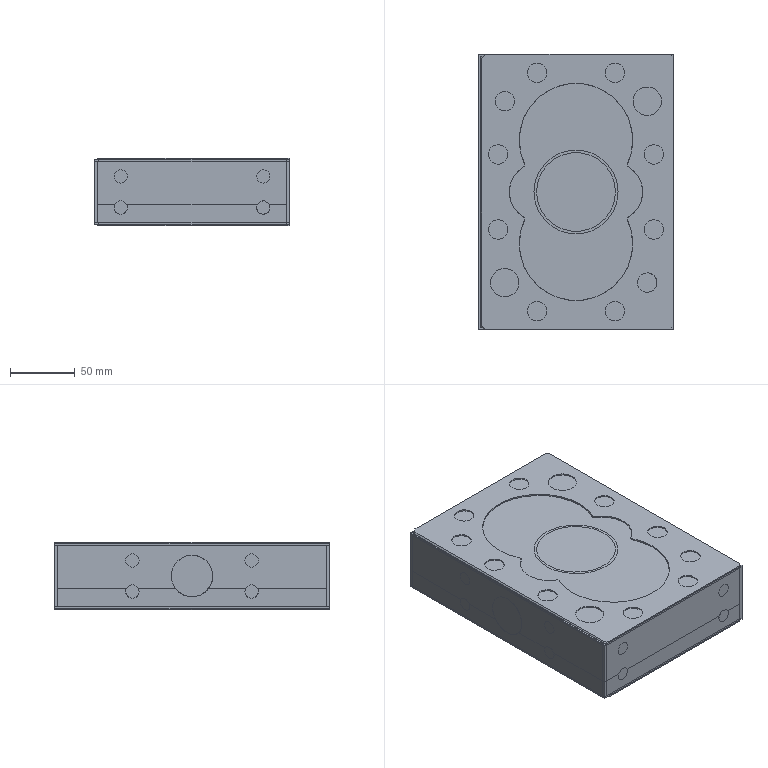NC program | NX | posted with a generic post | part box 150.2 x 212.2 x 52.4 mm
Lines 10319 to 11045 of 152230:
(孔铣开粗 , TOOL : D17R0.8圆鼻飞刀)
N20612 T03 M6
N20614 /M1
N20616 G54
N20618 G17 G0 G90 X-70. Y55. S1500 M3
N20620 G43 Z100. H3
N20622 Z1.2
N20624 G94 G1 Z0.2 F960.
N20626 G3 X-68.7 Y56.3 R1.3
N20628 X-70. Y57.6 R1.3
N20630 X-70. Y57.6 Z0. I0. J-2.6 F1200.
N20632 X-70. Y57.6 Z-0.2 I0. J-2.6
N20634 X-70. Y57.6 Z-0.4 I0. J-2.6
N20636 X-70. Y57.6 Z-0.6 I0. J-2.6
N20638 X-70. Y57.6 Z-0.8 I0. J-2.6
N20640 X-70. Y57.6 Z-1. I0. J-2.6
N20642 X-70. Y57.6 Z-1.2 I0. J-2.6
N20644 X-70. Y57.6 Z-1.4 I0. J-2.6
N20646 X-70. Y57.6 Z-1.6 I0. J-2.6
N20648 X-70. Y57.6 Z-1.8 I0. J-2.6
N20650 X-70. Y57.6 Z-2. I0. J-2.6
N20652 X-70. Y57.6 Z-2.2 I0. J-2.6
N20654 X-70. Y57.6 Z-2.4 I0. J-2.6
N20656 X-70. Y57.6 Z-2.6 I0. J-2.6
N20658 X-70. Y57.6 Z-2.8 I0. J-2.6
N20660 X-70. Y57.6 Z-3. I0. J-2.6
N20662 X-70. Y57.6 Z-3.2 I0. J-2.6
N20664 X-70. Y57.6 Z-3.4 I0. J-2.6
N20666 X-70. Y57.6 Z-3.6 I0. J-2.6
N20668 X-70. Y57.6 Z-3.8 I0. J-2.6
N20670 X-70. Y57.6 Z-4. I0. J-2.6
N20672 X-70. Y57.6 Z-4.2 I0. J-2.6
N20674 X-70. Y57.6 Z-4.4 I0. J-2.6
N20676 X-70. Y57.6 Z-4.6 I0. J-2.6
N20678 X-70. Y57.6 Z-4.8 I0. J-2.6
N20680 X-70. Y57.6 Z-5. I0. J-2.6
N20682 X-70. Y57.6 Z-5.2 I0. J-2.6
N20684 X-70. Y57.6 Z-5.4 I0. J-2.6
N20686 X-70. Y57.6 Z-5.6 I0. J-2.6
N20688 X-70. Y57.6 Z-5.8 I0. J-2.6
N20690 X-70. Y57.6 Z-6. I0. J-2.6
N20692 X-70. Y57.6 Z-6.2 I0. J-2.6
N20694 X-70. Y57.6 Z-6.4 I0. J-2.6
N20696 X-70. Y57.6 Z-6.6 I0. J-2.6
N20698 X-70. Y57.6 Z-6.8 I0. J-2.6
N20700 X-70. Y57.6 Z-7. I0. J-2.6
N20702 X-70. Y57.6 Z-7.2 I0. J-2.6
N20704 X-70. Y57.6 Z-7.4 I0. J-2.6
N20706 X-70. Y57.6 Z-7.6 I0. J-2.6
N20708 X-70. Y57.6 Z-7.8 I0. J-2.6
N20710 X-70. Y57.6 Z-8. I0. J-2.6
N20712 X-70. Y57.6 Z-8.2 I0. J-2.6
N20714 X-70. Y57.6 Z-8.4 I0. J-2.6
N20716 X-70. Y57.6 Z-8.6 I0. J-2.6
N20718 X-70. Y57.6 Z-8.8 I0. J-2.6
N20720 X-70. Y57.6 Z-9. I0. J-2.6
N20722 X-70. Y57.6 Z-9.2 I0. J-2.6
N20724 X-70. Y57.6 Z-9.4 I0. J-2.6
N20726 X-70. Y57.6 Z-9.6 I0. J-2.6
N20728 X-70. Y57.6 Z-9.8 I0. J-2.6
N20730 X-70. Y57.6 Z-10. I0. J-2.6
N20732 X-70. Y57.6 Z-10.2 I0. J-2.6
N20734 X-70. Y57.6 Z-10.4 I0. J-2.6
N20736 X-70. Y57.6 Z-10.6 I0. J-2.6
N20738 X-70. Y57.6 Z-10.8 I0. J-2.6
N20740 X-70. Y57.6 Z-11. I0. J-2.6
N20742 X-70. Y57.6 Z-11.2 I0. J-2.6
N20744 X-70. Y57.6 Z-11.4 I0. J-2.6
N20746 X-70. Y57.6 Z-11.6 I0. J-2.6
N20748 X-70. Y57.6 Z-11.8 I0. J-2.6
N20750 X-70. Y57.6 Z-12. I0. J-2.6
N20752 X-70. Y57.6 Z-12.2 I0. J-2.6
N20754 X-70. Y57.6 Z-12.4 I0. J-2.6
N20756 X-70. Y57.6 Z-12.6 I0. J-2.6
N20758 X-70. Y57.6 Z-12.8 I0. J-2.6
N20760 X-70. Y57.6 Z-13. I0. J-2.6
N20762 X-70. Y57.6 Z-13.2 I0. J-2.6
N20764 X-70. Y57.6 Z-13.4 I0. J-2.6
N20766 X-70. Y57.6 Z-13.6 I0. J-2.6
N20768 X-70. Y57.6 Z-13.8 I0. J-2.6
N20770 X-70. Y57.6 Z-14. I0. J-2.6
N20772 X-70. Y57.6 Z-14.2 I0. J-2.6
N20774 X-70. Y57.6 Z-14.4 I0. J-2.6
N20776 X-70. Y57.6 Z-14.6 I0. J-2.6
N20778 X-70. Y57.6 Z-14.8 I0. J-2.6
N20780 X-70. Y57.6 Z-15. I0. J-2.6
N20782 X-70. Y57.6 Z-15.2 I0. J-2.6
N20784 X-70. Y57.6 Z-15.4 I0. J-2.6
N20786 X-70. Y57.6 Z-15.6 I0. J-2.6
N20788 X-70. Y57.6 Z-15.8 I0. J-2.6
N20790 X-70. Y57.6 Z-16. I0. J-2.6
N20792 X-70. Y57.6 Z-16.2 I0. J-2.6
N20794 X-70. Y57.6 Z-16.4 I0. J-2.6
N20796 X-70. Y57.6 Z-16.6 I0. J-2.6
N20798 X-70. Y57.6 Z-16.8 I0. J-2.6
N20800 X-70. Y57.6 Z-17. I0. J-2.6
N20802 X-70. Y57.6 Z-17.2 I0. J-2.6
N20804 X-70. Y57.6 Z-17.4 I0. J-2.6
N20806 X-70. Y57.6 Z-17.6 I0. J-2.6
N20808 X-70. Y57.6 Z-17.8 I0. J-2.6
N20810 X-70. Y57.6 Z-18. I0. J-2.6
N20812 X-70. Y57.6 Z-18.2 I0. J-2.6
N20814 X-70. Y57.6 Z-18.4 I0. J-2.6
N20816 X-70. Y57.6 Z-18.6 I0. J-2.6
N20818 X-70. Y57.6 Z-18.8 I0. J-2.6
N20820 X-70. Y57.6 Z-19. I0. J-2.6
N20822 X-70. Y57.6 Z-19.2 I0. J-2.6
N20824 X-70. Y57.6 Z-19.4 I0. J-2.6
N20826 X-70. Y57.6 Z-19.6 I0. J-2.6
N20828 X-70. Y57.6 Z-19.8 I0. J-2.6
N20830 X-70. Y57.6 Z-20. I0. J-2.6
N20832 X-70. Y57.6 Z-20.2 I0. J-2.6
N20834 X-70. Y57.6 Z-20.4 I0. J-2.6
N20836 X-70. Y57.6 Z-20.6 I0. J-2.6
N20838 X-70. Y57.6 Z-20.8 I0. J-2.6
N20840 X-70. Y57.6 Z-21. I0. J-2.6
N20842 X-70. Y57.6 Z-21.2 I0. J-2.6
N20844 X-70. Y57.6 Z-21.4 I0. J-2.6
N20846 X-70. Y57.6 Z-21.6 I0. J-2.6
N20848 X-70. Y57.6 Z-21.8 I0. J-2.6
N20850 X-70. Y57.6 Z-22. I0. J-2.6
N20852 X-70. Y57.6 Z-22.2 I0. J-2.6
N20854 X-70. Y57.6 Z-22.4 I0. J-2.6
N20856 X-70. Y57.6 Z-22.6 I0. J-2.6
N20858 X-70. Y57.6 Z-22.8 I0. J-2.6
N20860 X-70. Y57.6 Z-23. I0. J-2.6
N20862 X-70. Y57.6 Z-23.2 I0. J-2.6
N20864 X-70. Y57.6 Z-23.4 I0. J-2.6
N20866 X-70. Y57.6 Z-23.6 I0. J-2.6
N20868 X-70. Y57.6 Z-23.8 I0. J-2.6
N20870 X-70. Y57.6 Z-24. I0. J-2.6
N20872 X-70. Y57.6 Z-24.2 I0. J-2.6
N20874 X-70. Y57.6 Z-24.4 I0. J-2.6
N20876 X-70. Y57.6 Z-24.6 I0. J-2.6
N20878 X-70. Y57.6 Z-24.8 I0. J-2.6
N20880 X-70. Y57.6 Z-25. I0. J-2.6
N20882 X-70. Y57.6 Z-25.2 I0. J-2.6
N20884 X-70. Y57.6 Z-25.4 I0. J-2.6
N20886 X-70. Y57.6 Z-25.6 I0. J-2.6
N20888 X-70. Y57.6 Z-25.8 I0. J-2.6
N20890 X-70. Y57.6 Z-26. I0. J-2.6
N20892 X-70. Y57.6 Z-26.2 I0. J-2.6
N20894 X-70. Y57.6 Z-26.4 I0. J-2.6
N20896 X-70. Y57.6 Z-26.6 I0. J-2.6
N20898 X-70. Y57.6 Z-26.8 I0. J-2.6
N20900 X-70. Y57.6 Z-27. I0. J-2.6
N20902 X-70. Y57.6 Z-27.2 I0. J-2.6
N20904 X-70. Y57.6 Z-27.4 I0. J-2.6
N20906 X-70. Y57.6 Z-27.6 I0. J-2.6
N20908 X-70. Y57.6 Z-27.8 I0. J-2.6
N20910 X-70. Y57.6 Z-28. I0. J-2.6
N20912 X-70. Y57.6 Z-28.2 I0. J-2.6
N20914 X-70. Y57.6 Z-28.4 I0. J-2.6
N20916 X-70. Y57.6 Z-28.6 I0. J-2.6
N20918 X-70. Y57.6 Z-28.8 I0. J-2.6
N20920 X-70. Y57.6 Z-29. I0. J-2.6
N20922 X-70. Y57.6 Z-29.2 I0. J-2.6
N20924 X-70. Y57.6 Z-29.4 I0. J-2.6
N20926 X-70. Y57.6 Z-29.6 I0. J-2.6
N20928 X-70. Y57.6 Z-29.8 I0. J-2.6
N20930 X-70. Y57.6 Z-30. I0. J-2.6
N20932 X-70. Y57.6 Z-30.2 I0. J-2.6
N20934 X-70. Y57.6 Z-30.4 I0. J-2.6
N20936 X-70. Y57.6 Z-30.6 I0. J-2.6
N20938 X-70. Y57.6 Z-30.8 I0. J-2.6
N20940 X-70. Y57.6 Z-31. I0. J-2.6
N20942 X-70. Y57.6 Z-31.2 I0. J-2.6
N20944 X-70. Y57.6 Z-31.4 I0. J-2.6
N20946 X-70. Y57.6 Z-31.6 I0. J-2.6
N20948 X-70. Y57.6 Z-31.8 I0. J-2.6
N20950 X-70. Y57.6 Z-32. I0. J-2.6
N20952 X-70. Y57.6 Z-32.2 I0. J-2.6
N20954 X-70. Y57.6 Z-32.4 I0. J-2.6
N20956 X-70. Y57.6 Z-32.6 I0. J-2.6
N20958 X-70. Y57.6 Z-32.8 I0. J-2.6
N20960 X-70. Y57.6 Z-33. I0. J-2.6
N20962 X-70. Y57.6 Z-33.2 I0. J-2.6
N20964 X-70. Y57.6 Z-33.4 I0. J-2.6
N20966 X-70. Y57.6 Z-33.6 I0. J-2.6
N20968 X-70. Y57.6 Z-33.8 I0. J-2.6
N20970 X-70. Y57.6 Z-34. I0. J-2.6
N20972 X-70. Y57.6 Z-34.2 I0. J-2.6
N20974 X-70. Y57.6 Z-34.4 I0. J-2.6
N20976 X-70. Y57.6 Z-34.6 I0. J-2.6
N20978 X-70. Y57.6 Z-34.8 I0. J-2.6
N20980 X-70. Y57.6 Z-35. I0. J-2.6
N20982 X-72.6 Y55. R2.6
N20984 X-70. Y57.6 R-2.6
N20986 X-71.3 Y56.3 R1.3
N20988 X-70. Y55. R1.3
N20990 G0 Z100.
N20992 X70. Y-55.
N20994 Z1.2
N20996 G1 Z0.2 F960.
N20998 G3 X71.3 Y-53.7 R1.3
N21000 X70. Y-52.4 R1.3
N21002 X70. Y-52.4 Z0. I0. J-2.6 F1200.
N21004 X70. Y-52.4 Z-0.2 I0. J-2.6
N21006 X70. Y-52.4 Z-0.4 I0. J-2.6
N21008 X70. Y-52.4 Z-0.6 I0. J-2.6
N21010 X70. Y-52.4 Z-0.8 I0. J-2.6
N21012 X70. Y-52.4 Z-1. I0. J-2.6
N21014 X70. Y-52.4 Z-1.2 I0. J-2.6
N21016 X70. Y-52.4 Z-1.4 I0. J-2.6
N21018 X70. Y-52.4 Z-1.6 I0. J-2.6
N21020 X70. Y-52.4 Z-1.8 I0. J-2.6
N21022 X70. Y-52.4 Z-2. I0. J-2.6
N21024 X70. Y-52.4 Z-2.2 I0. J-2.6
N21026 X70. Y-52.4 Z-2.4 I0. J-2.6
N21028 X70. Y-52.4 Z-2.6 I0. J-2.6
N21030 X70. Y-52.4 Z-2.8 I0. J-2.6
N21032 X70. Y-52.4 Z-3. I0. J-2.6
N21034 X70. Y-52.4 Z-3.2 I0. J-2.6
N21036 X70. Y-52.4 Z-3.4 I0. J-2.6
N21038 X70. Y-52.4 Z-3.6 I0. J-2.6
N21040 X70. Y-52.4 Z-3.8 I0. J-2.6
N21042 X70. Y-52.4 Z-4. I0. J-2.6
N21044 X70. Y-52.4 Z-4.2 I0. J-2.6
N21046 X70. Y-52.4 Z-4.4 I0. J-2.6
N21048 X70. Y-52.4 Z-4.6 I0. J-2.6
N21050 X70. Y-52.4 Z-4.8 I0. J-2.6
N21052 X70. Y-52.4 Z-5. I0. J-2.6
N21054 X70. Y-52.4 Z-5.2 I0. J-2.6
N21056 X70. Y-52.4 Z-5.4 I0. J-2.6
N21058 X70. Y-52.4 Z-5.6 I0. J-2.6
N21060 X70. Y-52.4 Z-5.8 I0. J-2.6
N21062 X70. Y-52.4 Z-6. I0. J-2.6
N21064 X70. Y-52.4 Z-6.2 I0. J-2.6
N21066 X70. Y-52.4 Z-6.4 I0. J-2.6
N21068 X70. Y-52.4 Z-6.6 I0. J-2.6
N21070 X70. Y-52.4 Z-6.8 I0. J-2.6
N21072 X70. Y-52.4 Z-7. I0. J-2.6
N21074 X70. Y-52.4 Z-7.2 I0. J-2.6
N21076 X70. Y-52.4 Z-7.4 I0. J-2.6
N21078 X70. Y-52.4 Z-7.6 I0. J-2.6
N21080 X70. Y-52.4 Z-7.8 I0. J-2.6
N21082 X70. Y-52.4 Z-8. I0. J-2.6
N21084 X70. Y-52.4 Z-8.2 I0. J-2.6
N21086 X70. Y-52.4 Z-8.4 I0. J-2.6
N21088 X70. Y-52.4 Z-8.6 I0. J-2.6
N21090 X70. Y-52.4 Z-8.8 I0. J-2.6
N21092 X70. Y-52.4 Z-9. I0. J-2.6
N21094 X70. Y-52.4 Z-9.2 I0. J-2.6
N21096 X70. Y-52.4 Z-9.4 I0. J-2.6
N21098 X70. Y-52.4 Z-9.6 I0. J-2.6
N21100 X70. Y-52.4 Z-9.8 I0. J-2.6
N21102 X70. Y-52.4 Z-10. I0. J-2.6
N21104 X70. Y-52.4 Z-10.2 I0. J-2.6
N21106 X70. Y-52.4 Z-10.4 I0. J-2.6
N21108 X70. Y-52.4 Z-10.6 I0. J-2.6
N21110 X70. Y-52.4 Z-10.8 I0. J-2.6
N21112 X70. Y-52.4 Z-11. I0. J-2.6
N21114 X70. Y-52.4 Z-11.2 I0. J-2.6
N21116 X70. Y-52.4 Z-11.4 I0. J-2.6
N21118 X70. Y-52.4 Z-11.6 I0. J-2.6
N21120 X70. Y-52.4 Z-11.8 I0. J-2.6
N21122 X70. Y-52.4 Z-12. I0. J-2.6
N21124 X70. Y-52.4 Z-12.2 I0. J-2.6
N21126 X70. Y-52.4 Z-12.4 I0. J-2.6
N21128 X70. Y-52.4 Z-12.6 I0. J-2.6
N21130 X70. Y-52.4 Z-12.8 I0. J-2.6
N21132 X70. Y-52.4 Z-13. I0. J-2.6
N21134 X70. Y-52.4 Z-13.2 I0. J-2.6
N21136 X70. Y-52.4 Z-13.4 I0. J-2.6
N21138 X70. Y-52.4 Z-13.6 I0. J-2.6
N21140 X70. Y-52.4 Z-13.8 I0. J-2.6
N21142 X70. Y-52.4 Z-14. I0. J-2.6
N21144 X70. Y-52.4 Z-14.2 I0. J-2.6
N21146 X70. Y-52.4 Z-14.4 I0. J-2.6
N21148 X70. Y-52.4 Z-14.6 I0. J-2.6
N21150 X70. Y-52.4 Z-14.8 I0. J-2.6
N21152 X70. Y-52.4 Z-15. I0. J-2.6
N21154 X70. Y-52.4 Z-15.2 I0. J-2.6
N21156 X70. Y-52.4 Z-15.4 I0. J-2.6
N21158 X70. Y-52.4 Z-15.6 I0. J-2.6
N21160 X70. Y-52.4 Z-15.8 I0. J-2.6
N21162 X70. Y-52.4 Z-16. I0. J-2.6
N21164 X70. Y-52.4 Z-16.2 I0. J-2.6
N21166 X70. Y-52.4 Z-16.4 I0. J-2.6
N21168 X70. Y-52.4 Z-16.6 I0. J-2.6
N21170 X70. Y-52.4 Z-16.8 I0. J-2.6
N21172 X70. Y-52.4 Z-17. I0. J-2.6
N21174 X70. Y-52.4 Z-17.2 I0. J-2.6
N21176 X70. Y-52.4 Z-17.4 I0. J-2.6
N21178 X70. Y-52.4 Z-17.6 I0. J-2.6
N21180 X70. Y-52.4 Z-17.8 I0. J-2.6
N21182 X70. Y-52.4 Z-18. I0. J-2.6
N21184 X70. Y-52.4 Z-18.2 I0. J-2.6
N21186 X70. Y-52.4 Z-18.4 I0. J-2.6
N21188 X70. Y-52.4 Z-18.6 I0. J-2.6
N21190 X70. Y-52.4 Z-18.8 I0. J-2.6
N21192 X70. Y-52.4 Z-19. I0. J-2.6
N21194 X70. Y-52.4 Z-19.2 I0. J-2.6
N21196 X70. Y-52.4 Z-19.4 I0. J-2.6
N21198 X70. Y-52.4 Z-19.6 I0. J-2.6
N21200 X70. Y-52.4 Z-19.8 I0. J-2.6
N21202 X70. Y-52.4 Z-20. I0. J-2.6
N21204 X70. Y-52.4 Z-20.2 I0. J-2.6
N21206 X70. Y-52.4 Z-20.4 I0. J-2.6
N21208 X70. Y-52.4 Z-20.6 I0. J-2.6
N21210 X70. Y-52.4 Z-20.8 I0. J-2.6
N21212 X70. Y-52.4 Z-21. I0. J-2.6
N21214 X70. Y-52.4 Z-21.2 I0. J-2.6
N21216 X70. Y-52.4 Z-21.4 I0. J-2.6
N21218 X70. Y-52.4 Z-21.6 I0. J-2.6
N21220 X70. Y-52.4 Z-21.8 I0. J-2.6
N21222 X70. Y-52.4 Z-22. I0. J-2.6
N21224 X70. Y-52.4 Z-22.2 I0. J-2.6
N21226 X70. Y-52.4 Z-22.4 I0. J-2.6
N21228 X70. Y-52.4 Z-22.6 I0. J-2.6
N21230 X70. Y-52.4 Z-22.8 I0. J-2.6
N21232 X70. Y-52.4 Z-23. I0. J-2.6
N21234 X70. Y-52.4 Z-23.2 I0. J-2.6
N21236 X70. Y-52.4 Z-23.4 I0. J-2.6
N21238 X70. Y-52.4 Z-23.6 I0. J-2.6
N21240 X70. Y-52.4 Z-23.8 I0. J-2.6
N21242 X70. Y-52.4 Z-24. I0. J-2.6
N21244 X70. Y-52.4 Z-24.2 I0. J-2.6
N21246 X70. Y-52.4 Z-24.4 I0. J-2.6
N21248 X70. Y-52.4 Z-24.6 I0. J-2.6
N21250 X70. Y-52.4 Z-24.8 I0. J-2.6
N21252 X70. Y-52.4 Z-25. I0. J-2.6
N21254 X70. Y-52.4 Z-25.2 I0. J-2.6
N21256 X70. Y-52.4 Z-25.4 I0. J-2.6
N21258 X70. Y-52.4 Z-25.6 I0. J-2.6
N21260 X70. Y-52.4 Z-25.8 I0. J-2.6
N21262 X70. Y-52.4 Z-26. I0. J-2.6
N21264 X70. Y-52.4 Z-26.2 I0. J-2.6
N21266 X70. Y-52.4 Z-26.4 I0. J-2.6
N21268 X70. Y-52.4 Z-26.6 I0. J-2.6
N21270 X70. Y-52.4 Z-26.8 I0. J-2.6
N21272 X70. Y-52.4 Z-27. I0. J-2.6
N21274 X70. Y-52.4 Z-27.2 I0. J-2.6
N21276 X70. Y-52.4 Z-27.4 I0. J-2.6
N21278 X70. Y-52.4 Z-27.6 I0. J-2.6
N21280 X70. Y-52.4 Z-27.8 I0. J-2.6
N21282 X70. Y-52.4 Z-28. I0. J-2.6
N21284 X70. Y-52.4 Z-28.2 I0. J-2.6
N21286 X70. Y-52.4 Z-28.4 I0. J-2.6
N21288 X70. Y-52.4 Z-28.6 I0. J-2.6
N21290 X70. Y-52.4 Z-28.8 I0. J-2.6
N21292 X70. Y-52.4 Z-29. I0. J-2.6
N21294 X70. Y-52.4 Z-29.2 I0. J-2.6
N21296 X70. Y-52.4 Z-29.4 I0. J-2.6
N21298 X70. Y-52.4 Z-29.6 I0. J-2.6
N21300 X70. Y-52.4 Z-29.8 I0. J-2.6
N21302 X70. Y-52.4 Z-30. I0. J-2.6
N21304 X70. Y-52.4 Z-30.2 I0. J-2.6
N21306 X70. Y-52.4 Z-30.4 I0. J-2.6
N21308 X70. Y-52.4 Z-30.6 I0. J-2.6
N21310 X70. Y-52.4 Z-30.8 I0. J-2.6
N21312 X70. Y-52.4 Z-31. I0. J-2.6
N21314 X70. Y-52.4 Z-31.2 I0. J-2.6
N21316 X70. Y-52.4 Z-31.4 I0. J-2.6
N21318 X70. Y-52.4 Z-31.6 I0. J-2.6
N21320 X70. Y-52.4 Z-31.8 I0. J-2.6
N21322 X70. Y-52.4 Z-32. I0. J-2.6
N21324 X70. Y-52.4 Z-32.2 I0. J-2.6
N21326 X70. Y-52.4 Z-32.4 I0. J-2.6
N21328 X70. Y-52.4 Z-32.6 I0. J-2.6
N21330 X70. Y-52.4 Z-32.8 I0. J-2.6
N21332 X70. Y-52.4 Z-33. I0. J-2.6
N21334 X70. Y-52.4 Z-33.2 I0. J-2.6
N21336 X70. Y-52.4 Z-33.4 I0. J-2.6
N21338 X70. Y-52.4 Z-33.6 I0. J-2.6
N21340 X70. Y-52.4 Z-33.8 I0. J-2.6
N21342 X70. Y-52.4 Z-34. I0. J-2.6
N21344 X70. Y-52.4 Z-34.2 I0. J-2.6
N21346 X70. Y-52.4 Z-34.4 I0. J-2.6
N21348 X70. Y-52.4 Z-34.6 I0. J-2.6
N21350 X70. Y-52.4 Z-34.8 I0. J-2.6
N21352 X70. Y-52.4 Z-35. I0. J-2.6
N21354 X67.4 Y-55. R2.6
N21356 X70. Y-52.4 R-2.6
N21358 X68.7 Y-53.7 R1.3
N21360 X70. Y-55. R1.3
N21362 G0 Z100.
(孔铣开粗_1 , TOOL : D17R0.8圆鼻飞刀)
N21364 /M1
N21366 X-70. Y55.
N21368 Z-33.8
N21370 G1 Z-34.8 F640.
N21372 G3 X-69.1 Y55.9 R0.9
N21374 X-70. Y56.8 R0.9
N21376 X-70. Y56.8 Z-35. I0. J-1.8 F800.
N21378 X-70. Y56.8 Z-35.2 I0. J-1.8
N21380 X-70. Y56.8 Z-35.4 I0. J-1.8
N21382 X-70. Y56.8 Z-35.6 I0. J-1.8
N21384 X-70. Y56.8 Z-35.8 I0. J-1.8
N21386 X-70. Y56.8 Z-36. I0. J-1.8
N21388 X-70. Y56.8 Z-36.2 I0. J-1.8
N21390 X-70. Y56.8 Z-36.4 I0. J-1.8
N21392 X-70. Y56.8 Z-36.6 I0. J-1.8
N21394 X-70. Y56.8 Z-36.8 I0. J-1.8
N21396 X-70. Y56.8 Z-37. I0. J-1.8
N21398 X-70. Y56.8 Z-37.2 I0. J-1.8
N21400 X-70. Y56.8 Z-37.4 I0. J-1.8
N21402 X-70. Y56.8 Z-37.6 I0. J-1.8
N21404 X-70. Y56.8 Z-37.8 I0. J-1.8
N21406 X-70. Y56.8 Z-38. I0. J-1.8
N21408 X-70. Y56.8 Z-38.2 I0. J-1.8
N21410 X-70. Y56.8 Z-38.4 I0. J-1.8
N21412 X-70. Y56.8 Z-38.6 I0. J-1.8
N21414 X-70. Y56.8 Z-38.8 I0. J-1.8
N21416 X-70. Y56.8 Z-39. I0. J-1.8
N21418 X-70. Y56.8 Z-39.2 I0. J-1.8
N21420 X-70. Y56.8 Z-39.4 I0. J-1.8
N21422 X-70. Y56.8 Z-39.6 I0. J-1.8
N21424 X-70. Y56.8 Z-39.8 I0. J-1.8
N21426 X-70. Y56.8 Z-40. I0. J-1.8
N21428 X-70. Y56.8 Z-40.2 I0. J-1.8
N21430 X-70. Y56.8 Z-40.4 I0. J-1.8
N21432 X-70. Y56.8 Z-40.6 I0. J-1.8
N21434 X-70. Y56.8 Z-40.8 I0. J-1.8
N21436 X-70. Y56.8 Z-41. I0. J-1.8
N21438 X-70. Y56.8 Z-41.2 I0. J-1.8
N21440 X-70. Y56.8 Z-41.4 I0. J-1.8
N21442 X-70. Y56.8 Z-41.6 I0. J-1.8
N21444 X-70. Y56.8 Z-41.8 I0. J-1.8
N21446 X-70. Y56.8 Z-42. I0. J-1.8
N21448 X-70. Y56.8 Z-42.2 I0. J-1.8
N21450 X-70. Y56.8 Z-42.4 I0. J-1.8
N21452 X-70. Y56.8 Z-42.6 I0. J-1.8
N21454 X-70. Y56.8 Z-42.8 I0. J-1.8
N21456 X-70. Y56.8 Z-43. I0. J-1.8
N21458 X-70. Y56.8 Z-43.2 I0. J-1.8
N21460 X-70. Y56.8 Z-43.4 I0. J-1.8
N21462 X-70. Y56.8 Z-43.6 I0. J-1.8
N21464 X-70. Y56.8 Z-43.8 I0. J-1.8
N21466 X-70. Y56.8 Z-44. I0. J-1.8
N21468 X-70. Y56.8 Z-44.2 I0. J-1.8
N21470 X-70. Y56.8 Z-44.4 I0. J-1.8
N21472 X-70. Y56.8 Z-44.6 I0. J-1.8
N21474 X-70. Y56.8 Z-44.8 I0. J-1.8
N21476 X-70. Y56.8 Z-45. I0. J-1.8
N21478 X-70. Y56.8 Z-45.2 I0. J-1.8
N21480 X-70. Y56.8 Z-45.4 I0. J-1.8
N21482 X-70. Y56.8 Z-45.6 I0. J-1.8
N21484 X-70. Y56.8 Z-45.8 I0. J-1.8
N21486 X-70. Y56.8 Z-46. I0. J-1.8
N21488 X-70. Y56.8 Z-46.2 I0. J-1.8
N21490 X-70. Y56.8 Z-46.4 I0. J-1.8
N21492 X-70. Y56.8 Z-46.6 I0. J-1.8
N21494 X-70. Y56.8 Z-46.8 I0. J-1.8
N21496 X-70. Y56.8 Z-47. I0. J-1.8
N21498 X-70. Y56.8 Z-47.2 I0. J-1.8
N21500 X-70. Y56.8 Z-47.4 I0. J-1.8
N21502 X-70. Y56.8 Z-47.6 I0. J-1.8
N21504 X-70. Y56.8 Z-47.8 I0. J-1.8
N21506 X-70. Y56.8 Z-48. I0. J-1.8
N21508 X-70. Y56.8 Z-48.2 I0. J-1.8
N21510 X-70. Y56.8 Z-48.4 I0. J-1.8
N21512 X-70. Y56.8 Z-48.6 I0. J-1.8
N21514 X-70. Y56.8 Z-48.8 I0. J-1.8
N21516 X-70. Y56.8 Z-49. I0. J-1.8
N21518 X-70. Y56.8 Z-49.2 I0. J-1.8
N21520 X-70. Y56.8 Z-49.4 I0. J-1.8
N21522 X-70. Y56.8 Z-49.6 I0. J-1.8
N21524 X-70. Y56.8 Z-49.8 I0. J-1.8
N21526 X-70. Y56.8 Z-50. I0. J-1.8
N21528 X-70. Y56.8 Z-50.2 I0. J-1.8
N21530 X-70. Y56.8 Z-50.4 I0. J-1.8
N21532 X-70. Y56.8 Z-50.6 I0. J-1.8
N21534 X-70. Y56.8 Z-50.8 I0. J-1.8
N21536 X-70. Y56.8 Z-51. I0. J-1.8
N21538 X-70. Y56.8 Z-51.2 I0. J-1.8
N21540 X-70. Y56.8 Z-51.4 I0. J-1.8
N21542 X-71.8 Y55. R1.8
N21544 X-70. Y56.8 R-1.8
N21546 X-70.9 Y55.9 R0.9
N21548 X-70. Y55. R0.9
N21550 G0 Z100.
N21552 X70. Y-55.
N21554 Z-33.8
N21556 G1 Z-34.8 F640.
N21558 G3 X70.9 Y-54.1 R0.9
N21560 X70. Y-53.2 R0.9
N21562 X70. Y-53.2 Z-35. I0. J-1.8 F800.
N21564 X70. Y-53.2 Z-35.2 I0. J-1.8
N21566 X70. Y-53.2 Z-35.4 I0. J-1.8
N21568 X70. Y-53.2 Z-35.6 I0. J-1.8
N21570 X70. Y-53.2 Z-35.8 I0. J-1.8
N21572 X70. Y-53.2 Z-36. I0. J-1.8
N21574 X70. Y-53.2 Z-36.2 I0. J-1.8
N21576 X70. Y-53.2 Z-36.4 I0. J-1.8
N21578 X70. Y-53.2 Z-36.6 I0. J-1.8
N21580 X70. Y-53.2 Z-36.8 I0. J-1.8
N21582 X70. Y-53.2 Z-37. I0. J-1.8
N21584 X70. Y-53.2 Z-37.2 I0. J-1.8
N21586 X70. Y-53.2 Z-37.4 I0. J-1.8
N21588 X70. Y-53.2 Z-37.6 I0. J-1.8
N21590 X70. Y-53.2 Z-37.8 I0. J-1.8
N21592 X70. Y-53.2 Z-38. I0. J-1.8
N21594 X70. Y-53.2 Z-38.2 I0. J-1.8
N21596 X70. Y-53.2 Z-38.4 I0. J-1.8
N21598 X70. Y-53.2 Z-38.6 I0. J-1.8
N21600 X70. Y-53.2 Z-38.8 I0. J-1.8
N21602 X70. Y-53.2 Z-39. I0. J-1.8
N21604 X70. Y-53.2 Z-39.2 I0. J-1.8
N21606 X70. Y-53.2 Z-39.4 I0. J-1.8
N21608 X70. Y-53.2 Z-39.6 I0. J-1.8
N21610 X70. Y-53.2 Z-39.8 I0. J-1.8
N21612 X70. Y-53.2 Z-40. I0. J-1.8
N21614 X70. Y-53.2 Z-40.2 I0. J-1.8
N21616 X70. Y-53.2 Z-40.4 I0. J-1.8
N21618 X70. Y-53.2 Z-40.6 I0. J-1.8
N21620 X70. Y-53.2 Z-40.8 I0. J-1.8
N21622 X70. Y-53.2 Z-41. I0. J-1.8
N21624 X70. Y-53.2 Z-41.2 I0. J-1.8
N21626 X70. Y-53.2 Z-41.4 I0. J-1.8
N21628 X70. Y-53.2 Z-41.6 I0. J-1.8
N21630 X70. Y-53.2 Z-41.8 I0. J-1.8
N21632 X70. Y-53.2 Z-42. I0. J-1.8
N21634 X70. Y-53.2 Z-42.2 I0. J-1.8
N21636 X70. Y-53.2 Z-42.4 I0. J-1.8
N21638 X70. Y-53.2 Z-42.6 I0. J-1.8
N21640 X70. Y-53.2 Z-42.8 I0. J-1.8
N21642 X70. Y-53.2 Z-43. I0. J-1.8
N21644 X70. Y-53.2 Z-43.2 I0. J-1.8
N21646 X70. Y-53.2 Z-43.4 I0. J-1.8
N21648 X70. Y-53.2 Z-43.6 I0. J-1.8
N21650 X70. Y-53.2 Z-43.8 I0. J-1.8
N21652 X70. Y-53.2 Z-44. I0. J-1.8
N21654 X70. Y-53.2 Z-44.2 I0. J-1.8
N21656 X70. Y-53.2 Z-44.4 I0. J-1.8
N21658 X70. Y-53.2 Z-44.6 I0. J-1.8
N21660 X70. Y-53.2 Z-44.8 I0. J-1.8
N21662 X70. Y-53.2 Z-45. I0. J-1.8
N21664 X70. Y-53.2 Z-45.2 I0. J-1.8
N21666 X70. Y-53.2 Z-45.4 I0. J-1.8
N21668 X70. Y-53.2 Z-45.6 I0. J-1.8
N21670 X70. Y-53.2 Z-45.8 I0. J-1.8
N21672 X70. Y-53.2 Z-46. I0. J-1.8
N21674 X70. Y-53.2 Z-46.2 I0. J-1.8
N21676 X70. Y-53.2 Z-46.4 I0. J-1.8
N21678 X70. Y-53.2 Z-46.6 I0. J-1.8
N21680 X70. Y-53.2 Z-46.8 I0. J-1.8
N21682 X70. Y-53.2 Z-47. I0. J-1.8
N21684 X70. Y-53.2 Z-47.2 I0. J-1.8
N21686 X70. Y-53.2 Z-47.4 I0. J-1.8
N21688 X70. Y-53.2 Z-47.6 I0. J-1.8
N21690 X70. Y-53.2 Z-47.8 I0. J-1.8
N21692 X70. Y-53.2 Z-48. I0. J-1.8
N21694 X70. Y-53.2 Z-48.2 I0. J-1.8
N21696 X70. Y-53.2 Z-48.4 I0. J-1.8
N21698 X70. Y-53.2 Z-48.6 I0. J-1.8
N21700 X70. Y-53.2 Z-48.8 I0. J-1.8
N21702 X70. Y-53.2 Z-49. I0. J-1.8
N21704 X70. Y-53.2 Z-49.2 I0. J-1.8
N21706 X70. Y-53.2 Z-49.4 I0. J-1.8
N21708 X70. Y-53.2 Z-49.6 I0. J-1.8
N21710 X70. Y-53.2 Z-49.8 I0. J-1.8
N21712 X70. Y-53.2 Z-50. I0. J-1.8
N21714 X70. Y-53.2 Z-50.2 I0. J-1.8
N21716 X70. Y-53.2 Z-50.4 I0. J-1.8
N21718 X70. Y-53.2 Z-50.6 I0. J-1.8
N21720 X70. Y-53.2 Z-50.8 I0. J-1.8
N21722 X70. Y-53.2 Z-51. I0. J-1.8
N21724 X70. Y-53.2 Z-51.2 I0. J-1.8
N21726 X70. Y-53.2 Z-51.4 I0. J-1.8
N21728 X68.2 Y-55. R1.8
N21730 X70. Y-53.2 R-1.8
N21732 X69.1 Y-54.1 R0.9
N21734 X70. Y-55. R0.9
N21736 G0 Z100.
(等高外形 , TOOL : D17R0.8圆鼻飞刀)
N21738 /M1
N21740 X67.858 Y-16.724 S2750
N21742 Z0.202
N21744 G1 Z0.002 F2200.
N21746 G41 X67.955 Y-16.701 D3
N21748 G3 X73.71 Y-10.282 R10.2
N21750 X74.004 Y-9.263 R39.573 F2750.
N21752 X74.587 Y-6.791 R36.305
N21754 X75.168 Y-2.35 R36.903
N21756 G1 X75.17 Y-2.343
N21758 G3 X75.168 Y2.351 R37.466
N21760 X74.585 Y6.795 R36.679
N21762 X74.004 Y9.265 R35.893
N21764 G1 X73.873 Y9.727
N21766 G3 X73.419 Y11.198 R35.147
N21768 X72.837 Y12.796 R36.884
N21770 G1 X72.371 Y13.945
N21772 X72.254 Y14.202
N21774 G3 X71.673 Y15.459 R28.462
N21776 G1 X71.309 Y16.176
N21778 G3 X70.049 Y18.414 R29.663
N21780 X69.342 Y19.521 R17.562
N21782 G1 X68.935 Y20.122
N21784 G3 X68.175 Y21.171 R20.625
N21786 X67.789 Y21.68 R10.239
N21788 G1 X66.953 Y22.718
N21790 X66.089 Y23.697
N21792 G3 X65.421 Y24.408 R14.806
N21794 X64.253 Y25.569 R24.174
N21796 X62.274 Y27.31 R31.299
N21798 X60.767 Y28.474 R26.121
N21800 G1 X60.018 Y29.007
N21802 X59.941 Y29.058
N21804 G3 X58.141 Y30.216 R30.372
N21806 X57.131 Y30.797 R18.119
N21808 X56.041 Y31.379 R14.305
N21810 X54.856 Y31.959 R19.1
N21812 X53.543 Y32.537 R29.006
N21814 G1 X52.651 Y32.897
N21816 G3 X52.043 Y33.121 R10.15
N21818 X50.302 Y33.702 R26.55
N21820 X45.19 Y34.864 R34.769
N21822 X36.127 Y35.034 R35.529
N21824 G1 X34.805 Y34.865
N21826 X34.801 Y34.863
N21828 G3 X31.807 Y34.282 R40.11
N21830 X29.699 Y33.703 R34.573
N21832 G1 X29.695 Y33.701
N21834 G3 X27.96 Y33.124 R28.028
N21836 G1 X27.954 Y33.119
N21838 X27.667 Y33.021
N21840 X26.462 Y32.542
N21842 X26.455 Y32.538
N21844 X26.221 Y32.445
N21846 X25.145 Y31.961
N21848 X24.652 Y31.74
N21850 G2 X21.189 Y31.002 R8.442
N21852 G1 X20.413 Y31.004
N21854 X20.394 Y31.
N21856 X19.907
N21858 G2 X12.294 Y35.698 R8.52
N21860 G1 X12.235 Y35.788
N21862 G3 X11.654 Y36.746 R12.454
N21864 G1 X11.345 Y37.189
N21866 G3 X9.236 Y39.512 R13.562
N21868 X8.527 Y40.093 R9.941
N21870 X7.965 Y40.507 R7.187
N21872 G1 X7.711 Y40.674
N21874 X7.575 Y40.767
N21876 X6.758 Y41.256
N21878 G3 X5.565 Y41.837 R12.19
N21880 X3.964 Y42.418 R11.576
N21882 X-3.967 Y42.42 R13.911
N21884 G1 X-3.971 Y42.416
N21886 G3 X-5.568 Y41.839 R12.354
N21888 G1 X-5.573 Y41.835
N21890 G3 X-7.717 Y40.672 R13.49
N21892 G1 X-7.721 Y40.671
N21894 G3 X-8.528 Y40.096 R10.752
N21896 G1 X-8.532 Y40.091
N21898 G3 X-11.661 Y36.738 R13.715
N21900 X-12.235 Y35.788 R10.831
N21902 G1 X-12.344 Y35.608
N21904 G2 X-19.907 Y31. R8.505
N21906 G1 X-21.186
N21908 G2 X-24.613 Y31.723 R8.485
N21910 G1 X-24.845 Y31.825
N21912 X-25.052 Y31.911
N21914 X-25.147 Y31.961
N21916 X-26.221 Y32.445
N21918 X-26.456 Y32.538
N21920 X-26.462 Y32.541
N21922 X-27.668 Y33.02
N21924 X-27.957 Y33.122
N21926 G3 X-29.698 Y33.701 R26.648
N21928 X-31.813 Y34.285 R34.532
N21930 X-34.802 Y34.863 R40.61
N21932 G1 X-34.805 Y34.865
N21934 G3 X-39.041 Y35.233 R37.347
N21936 X-45.183 Y34.866 R35.818
N21938 G1 X-45.194 Y34.863
N21940 G3 X-48.947 Y34.088 R35.041
N21942 X-50.306 Y33.701 R19.034
N21944 X-52.047 Y33.119 R26.482
N21946 X-53.535 Y32.542 R27.798
N21948 G1 X-53.539 Y32.538
N21950 G3 X-54.862 Y31.956 R30.411
N21952 X-55.14 Y31.829 R4.769
N21954 G1 X-56.3 Y31.251
N21956 G3 X-57.129 Y30.8 R13.217
N21958 G1 X-57.134 Y30.795
N21960 G3 X-58.148 Y30.213 R18.459
N21962 X-59.949 Y29.052 R28.22
N21964 G1 X-60.773 Y28.47
N21966 G3 X-62.269 Y27.316 R27.137
N21968 G1 X-62.276 Y27.309
N21970 G3 X-64.255 Y25.568 R31.246
N21972 G1 X-64.825 Y25.016
N21974 G3 X-65.424 Y24.404 R16.417
N21976 X-66.139 Y23.643 R15.372
N21978 G1 X-66.997 Y22.665
N21980 X-67.834 Y21.625
N21982 G3 X-68.182 Y21.164 R8.566
N21984 X-68.965 Y20.079 R20.984
N21986 G1 X-69.576 Y19.175
N21988 G3 X-69.925 Y18.614 R8.922
N21990 X-71.675 Y15.458 R33.417
N21992 X-72.257 Y14.198 R28.204
N21994 G1 X-72.372 Y13.945
N21996 X-72.841 Y12.791
N21998 G3 X-73.42 Y11.198 R38.312
N22000 G1 X-73.424 Y11.188
N22002 G3 X-74.004 Y9.265 R38.448
N22004 X-74.585 Y6.795 R34.675
N22006 G1 X-74.588 Y6.791
N22008 G3 X-75.168 Y2.351 R36.697
N22010 G1 X-75.17 Y2.344
N22012 G3 X-75.168 Y-2.35 R37.123
N22014 X-74.585 Y-6.795 R36.351
N22016 X-74.003 Y-9.269 R34.301
N22018 X-73.42 Y-11.198 R36.14
N22020 X-72.836 Y-12.801 R36.117
N22022 G1 X-72.372 Y-13.945
N22024 X-72.259 Y-14.195
N22026 X-72.254 Y-14.201
N22028 G3 X-71.673 Y-15.459 R24.881
N22030 G1 X-71.381 Y-16.039
N22032 G3 X-70.506 Y-17.653 R30.813
N22034 G1 X-70.406 Y-17.834
N22036 X-69.927 Y-18.613
N22038 X-69.924 Y-18.615
N22040 G3 X-69.339 Y-19.525 R13.696
N22042 X-68.608 Y-20.585 R19.752
N22044 G1 X-67.936 Y-21.495
N22046 X-66.993 Y-22.675